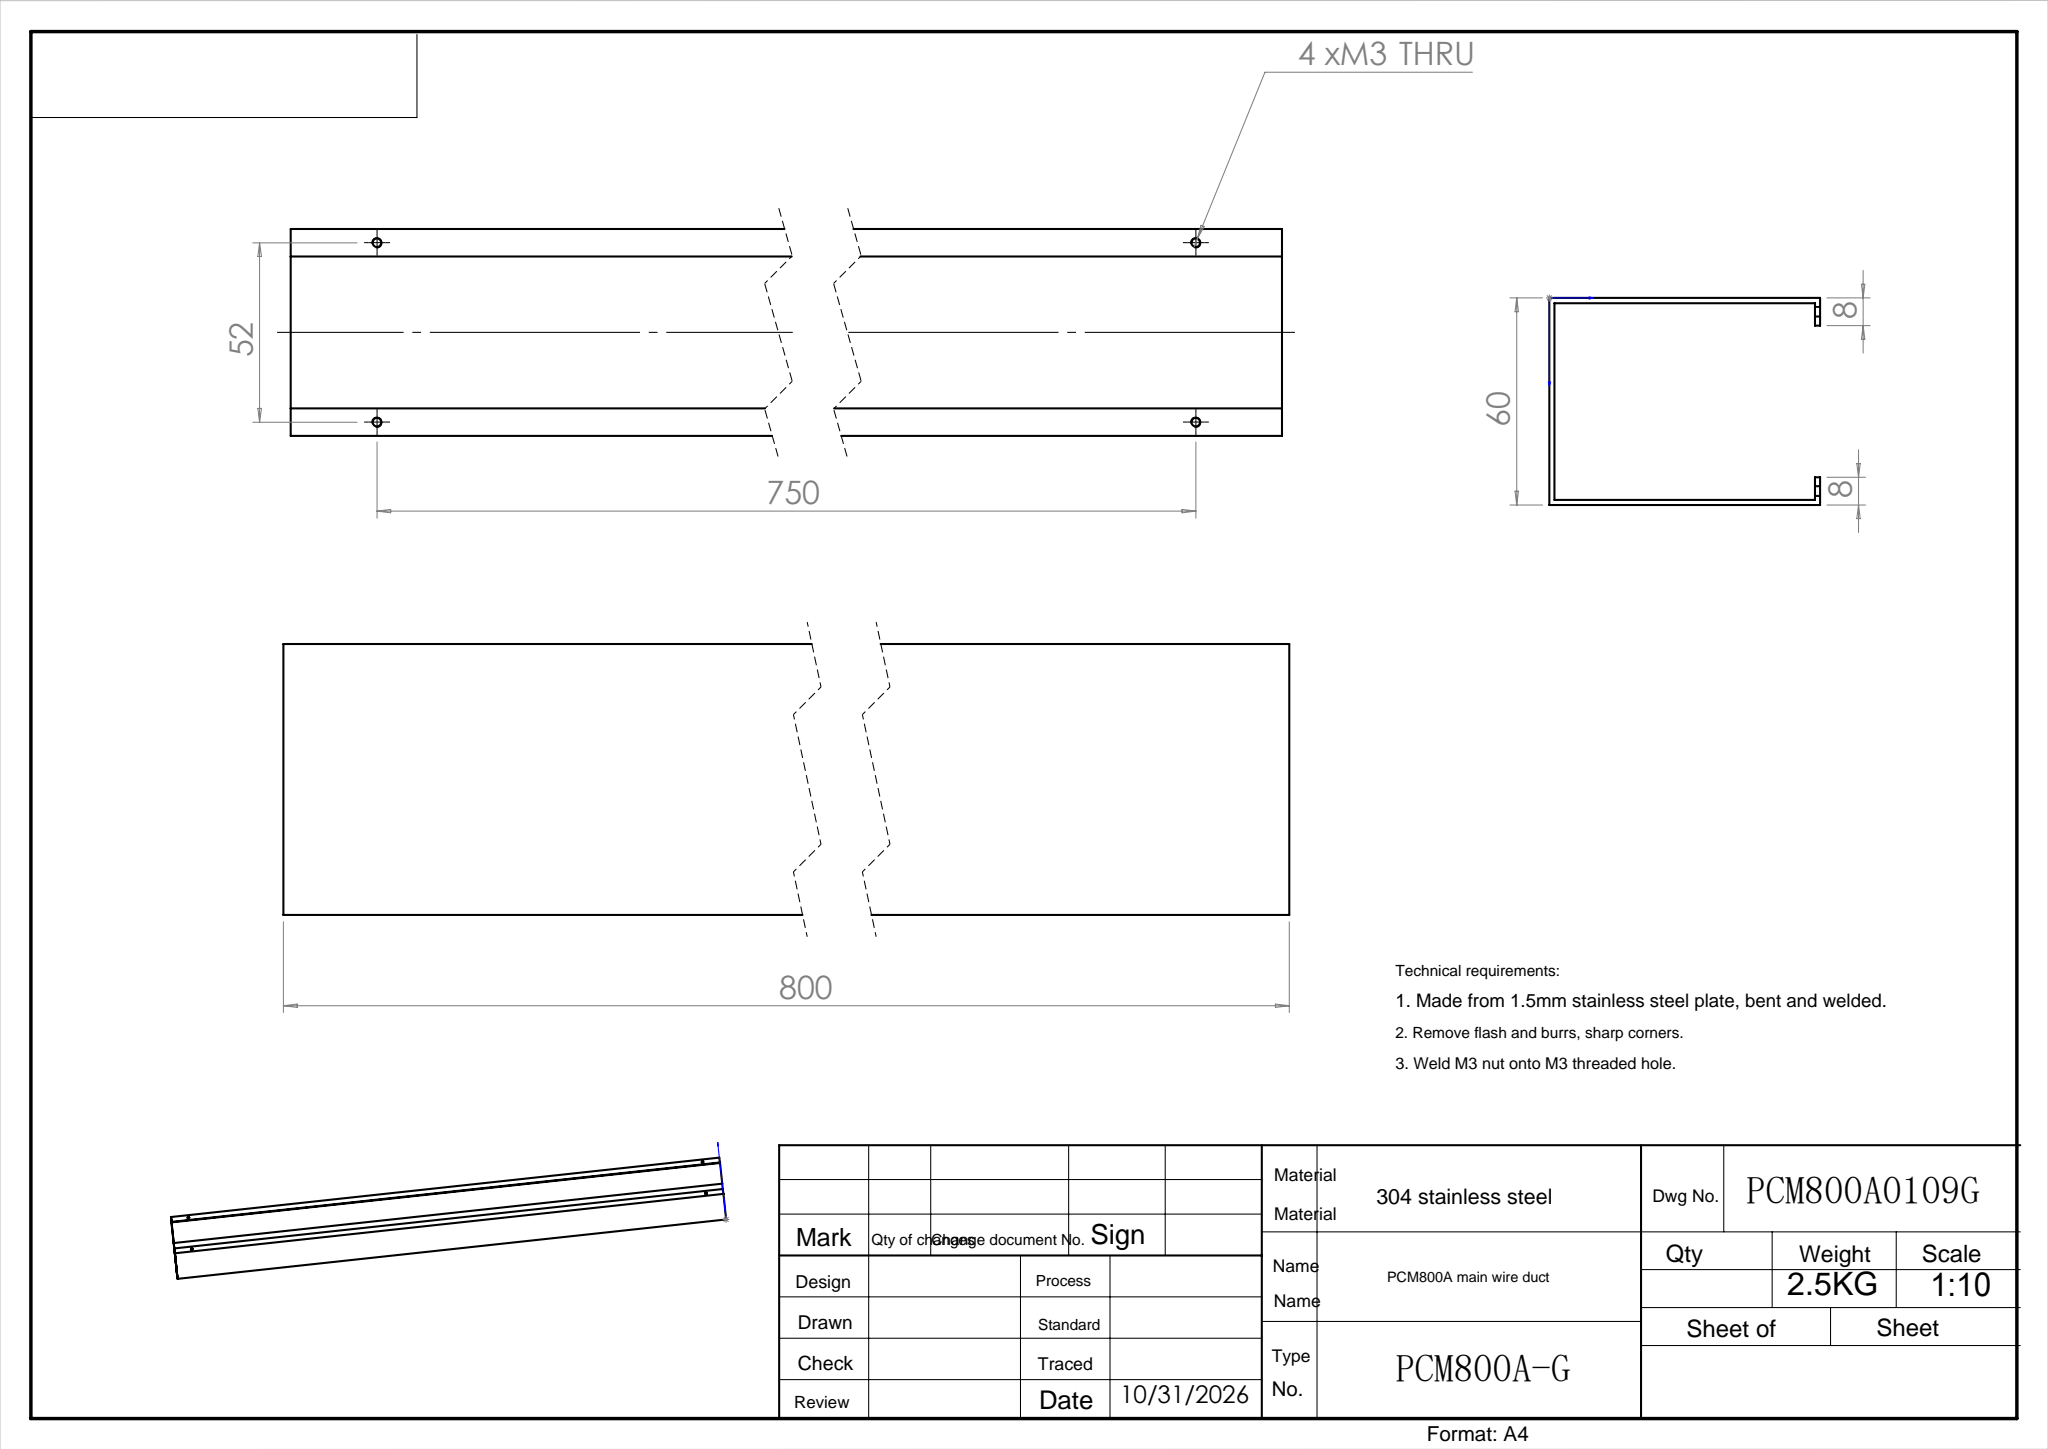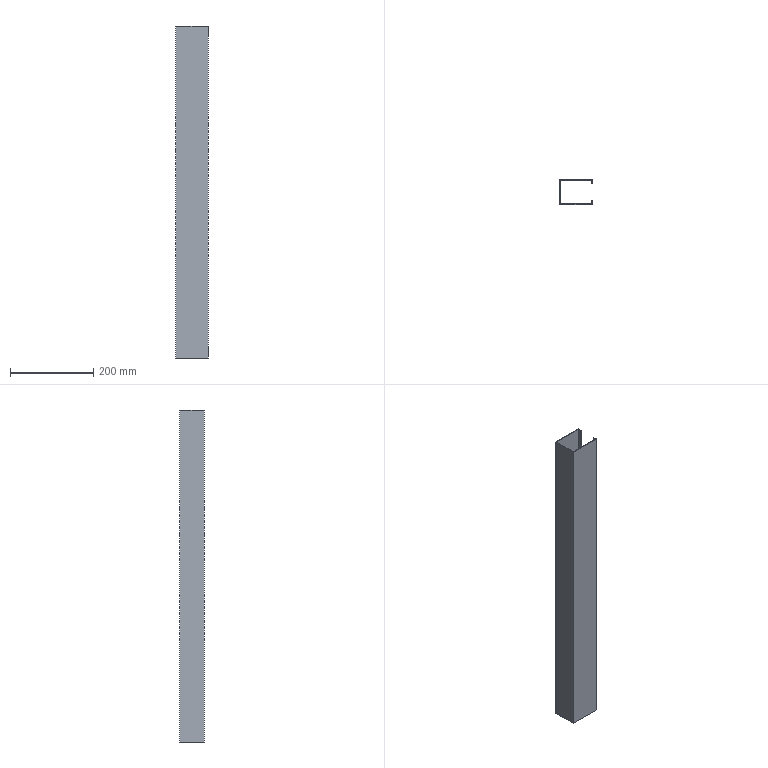Part | SolidWorks | features ExtruThin 1, HoleWzd 1, MirrorPattern 1 | 1 solid | 22 faces | box 78.5 x 60 x 800 mm | volume 272371 mm3 | plane 14 | cylinder 8 | commonest cylinder face diameters 2.5 x8
STEP:
#1=CARTESIAN_POINT('',(77.,4.,776.25));
#2=VERTEX_POINT('',#1);
#3=CARTESIAN_POINT('',(77.,4.,773.75));
#4=VERTEX_POINT('',#3);
#5=CARTESIAN_POINT('',(77.,4.,775.));
#6=DIRECTION('',(1.,0.,0.));
#7=DIRECTION('',(0.,0.,-1.));
#8=AXIS2_PLACEMENT_3D('',#5,#6,#7);
#9=CIRCLE('',#8,1.25);
#10=EDGE_CURVE('',#2,#4,#9,.T.);
#11=ORIENTED_EDGE('',*,*,#10,.F.);
#12=CARTESIAN_POINT('',(78.5,4.,776.25));
#13=VERTEX_POINT('',#12);
#14=CARTESIAN_POINT('',(78.5,4.,776.25));
#15=DIRECTION('',(1.,0.,0.));
#16=VECTOR('',#15,1000.);
#17=LINE('',#14,#16);
#18=EDGE_CURVE('',#2,#13,#17,.T.);
#19=ORIENTED_EDGE('',*,*,#18,.T.);
#20=CARTESIAN_POINT('',(78.5,4.,773.75));
#21=VERTEX_POINT('',#20);
#22=CARTESIAN_POINT('',(78.5,4.,775.));
#23=DIRECTION('',(1.,0.,0.));
#24=DIRECTION('',(0.,0.,-1.));
#25=AXIS2_PLACEMENT_3D('',#22,#23,#24);
#26=CIRCLE('',#25,1.25);
#27=EDGE_CURVE('',#13,#21,#26,.T.);
#28=ORIENTED_EDGE('',*,*,#27,.T.);
#29=CARTESIAN_POINT('',(78.5,4.,773.75));
#30=DIRECTION('',(1.,0.,0.));
#31=VECTOR('',#30,1000.);
#32=LINE('',#29,#31);
#33=EDGE_CURVE('',#4,#21,#32,.T.);
#34=ORIENTED_EDGE('',*,*,#33,.F.);
#35=EDGE_LOOP('',(#11,#19,#28,#34));
#36=FACE_OUTER_BOUND('',#35,.T.);
#37=CARTESIAN_POINT('',(78.5,4.,775.));
#38=DIRECTION('',(1.,0.,0.));
#39=DIRECTION('',(0.,0.,-1.));
#40=AXIS2_PLACEMENT_3D('',#37,#38,#39);
#41=CYLINDRICAL_SURFACE('',#40,1.25);
#42=ADVANCED_FACE('',(#36),#41,.F.);
#43=CARTESIAN_POINT('',(77.,4.,26.25));
#44=VERTEX_POINT('',#43);
#45=CARTESIAN_POINT('',(77.,4.,23.75));
#46=VERTEX_POINT('',#45);
#47=CARTESIAN_POINT('',(77.,4.,25.));
#48=DIRECTION('',(1.,0.,0.));
#49=DIRECTION('',(0.,0.,-1.));
#50=AXIS2_PLACEMENT_3D('',#47,#48,#49);
#51=CIRCLE('',#50,1.25);
#52=EDGE_CURVE('',#44,#46,#51,.T.);
#53=ORIENTED_EDGE('',*,*,#52,.F.);
#54=CARTESIAN_POINT('',(78.5,4.,26.25));
#55=VERTEX_POINT('',#54);
#56=CARTESIAN_POINT('',(78.5,4.,26.25));
#57=DIRECTION('',(1.,0.,0.));
#58=VECTOR('',#57,1000.);
#59=LINE('',#56,#58);
#60=EDGE_CURVE('',#44,#55,#59,.T.);
#61=ORIENTED_EDGE('',*,*,#60,.T.);
#62=CARTESIAN_POINT('',(78.5,4.,23.75));
#63=VERTEX_POINT('',#62);
#64=CARTESIAN_POINT('',(78.5,4.,25.));
#65=DIRECTION('',(1.,0.,0.));
#66=DIRECTION('',(0.,0.,-1.));
#67=AXIS2_PLACEMENT_3D('',#64,#65,#66);
#68=CIRCLE('',#67,1.25);
#69=EDGE_CURVE('',#55,#63,#68,.T.);
#70=ORIENTED_EDGE('',*,*,#69,.T.);
#71=CARTESIAN_POINT('',(78.5,4.,23.75));
#72=DIRECTION('',(1.,0.,0.));
#73=VECTOR('',#72,1000.);
#74=LINE('',#71,#73);
#75=EDGE_CURVE('',#46,#63,#74,.T.);
#76=ORIENTED_EDGE('',*,*,#75,.F.);
#77=EDGE_LOOP('',(#53,#61,#70,#76));
#78=FACE_OUTER_BOUND('',#77,.T.);
#79=CARTESIAN_POINT('',(78.5,4.,25.));
#80=DIRECTION('',(1.,0.,0.));
#81=DIRECTION('',(0.,0.,-1.));
#82=AXIS2_PLACEMENT_3D('',#79,#80,#81);
#83=CYLINDRICAL_SURFACE('',#82,1.25);
#84=ADVANCED_FACE('',(#78),#83,.F.);
#85=CARTESIAN_POINT('',(77.,56.,776.25));
#86=VERTEX_POINT('',#85);
#87=CARTESIAN_POINT('',(77.,56.,773.75));
#88=VERTEX_POINT('',#87);
#89=CARTESIAN_POINT('',(77.,56.,775.));
#90=DIRECTION('',(1.,0.,0.));
#91=DIRECTION('',(0.,1.,0.));
#92=AXIS2_PLACEMENT_3D('',#89,#90,#91);
#93=CIRCLE('',#92,1.25);
#94=EDGE_CURVE('',#86,#88,#93,.T.);
#95=ORIENTED_EDGE('',*,*,#94,.F.);
#96=CARTESIAN_POINT('',(78.5,56.,776.25));
#97=VERTEX_POINT('',#96);
#98=CARTESIAN_POINT('',(78.5,56.,776.25));
#99=DIRECTION('',(1.,0.,0.));
#100=VECTOR('',#99,1000.);
#101=LINE('',#98,#100);
#102=EDGE_CURVE('',#86,#97,#101,.T.);
#103=ORIENTED_EDGE('',*,*,#102,.T.);
#104=CARTESIAN_POINT('',(78.5,56.,773.75));
#105=VERTEX_POINT('',#104);
#106=CARTESIAN_POINT('',(78.5,56.,775.));
#107=DIRECTION('',(1.,0.,0.));
#108=DIRECTION('',(0.,0.,-1.));
#109=AXIS2_PLACEMENT_3D('',#106,#107,#108);
#110=CIRCLE('',#109,1.25);
#111=EDGE_CURVE('',#97,#105,#110,.T.);
#112=ORIENTED_EDGE('',*,*,#111,.T.);
#113=CARTESIAN_POINT('',(78.5,56.,773.75));
#114=DIRECTION('',(1.,0.,0.));
#115=VECTOR('',#114,1000.);
#116=LINE('',#113,#115);
#117=EDGE_CURVE('',#88,#105,#116,.T.);
#118=ORIENTED_EDGE('',*,*,#117,.F.);
#119=EDGE_LOOP('',(#95,#103,#112,#118));
#120=FACE_OUTER_BOUND('',#119,.T.);
#121=CARTESIAN_POINT('',(78.5,56.,775.));
#122=DIRECTION('',(1.,0.,0.));
#123=DIRECTION('',(0.,0.,-1.));
#124=AXIS2_PLACEMENT_3D('',#121,#122,#123);
#125=CYLINDRICAL_SURFACE('',#124,1.25);
#126=ADVANCED_FACE('',(#120),#125,.F.);
#127=CARTESIAN_POINT('',(77.,56.,26.25));
#128=VERTEX_POINT('',#127);
#129=CARTESIAN_POINT('',(77.,56.,23.75));
#130=VERTEX_POINT('',#129);
#131=CARTESIAN_POINT('',(77.,56.,25.));
#132=DIRECTION('',(1.,0.,0.));
#133=DIRECTION('',(0.,1.,0.));
#134=AXIS2_PLACEMENT_3D('',#131,#132,#133);
#135=CIRCLE('',#134,1.25);
#136=EDGE_CURVE('',#128,#130,#135,.T.);
#137=ORIENTED_EDGE('',*,*,#136,.F.);
#138=CARTESIAN_POINT('',(78.5,56.,26.25));
#139=VERTEX_POINT('',#138);
#140=CARTESIAN_POINT('',(78.5,56.,26.25));
#141=DIRECTION('',(1.,0.,0.));
#142=VECTOR('',#141,1000.);
#143=LINE('',#140,#142);
#144=EDGE_CURVE('',#128,#139,#143,.T.);
#145=ORIENTED_EDGE('',*,*,#144,.T.);
#146=CARTESIAN_POINT('',(78.5,56.,23.75));
#147=VERTEX_POINT('',#146);
#148=CARTESIAN_POINT('',(78.5,56.,25.));
#149=DIRECTION('',(1.,0.,0.));
#150=DIRECTION('',(0.,0.,-1.));
#151=AXIS2_PLACEMENT_3D('',#148,#149,#150);
#152=CIRCLE('',#151,1.25);
#153=EDGE_CURVE('',#139,#147,#152,.T.);
#154=ORIENTED_EDGE('',*,*,#153,.T.);
#155=CARTESIAN_POINT('',(78.5,56.,23.75));
#156=DIRECTION('',(1.,0.,0.));
#157=VECTOR('',#156,1000.);
#158=LINE('',#155,#157);
#159=EDGE_CURVE('',#130,#147,#158,.T.);
#160=ORIENTED_EDGE('',*,*,#159,.F.);
#161=EDGE_LOOP('',(#137,#145,#154,#160));
#162=FACE_OUTER_BOUND('',#161,.T.);
#163=CARTESIAN_POINT('',(78.5,56.,25.));
#164=DIRECTION('',(1.,0.,0.));
#165=DIRECTION('',(0.,0.,-1.));
#166=AXIS2_PLACEMENT_3D('',#163,#164,#165);
#167=CYLINDRICAL_SURFACE('',#166,1.25);
#168=ADVANCED_FACE('',(#162),#167,.F.);
#169=CARTESIAN_POINT('',(77.,56.,775.));
#170=DIRECTION('',(1.,0.,0.));
#171=DIRECTION('',(0.,1.,0.));
#172=AXIS2_PLACEMENT_3D('',#169,#170,#171);
#173=CIRCLE('',#172,1.25);
#174=EDGE_CURVE('',#88,#86,#173,.T.);
#175=ORIENTED_EDGE('',*,*,#174,.T.);
#176=ORIENTED_EDGE('',*,*,#94,.T.);
#177=EDGE_LOOP('',(#175,#176));
#178=FACE_BOUND('',#177,.T.);
#179=CARTESIAN_POINT('',(77.,56.,25.));
#180=DIRECTION('',(1.,0.,0.));
#181=DIRECTION('',(0.,1.,0.));
#182=AXIS2_PLACEMENT_3D('',#179,#180,#181);
#183=CIRCLE('',#182,1.25);
#184=EDGE_CURVE('',#130,#128,#183,.T.);
#185=ORIENTED_EDGE('',*,*,#184,.T.);
#186=ORIENTED_EDGE('',*,*,#136,.T.);
#187=EDGE_LOOP('',(#185,#186));
#188=FACE_BOUND('',#187,.T.);
#189=CARTESIAN_POINT('',(77.,58.5,0.));
#190=VERTEX_POINT('',#189);
#191=CARTESIAN_POINT('',(77.,52.,0.));
#192=VERTEX_POINT('',#191);
#193=CARTESIAN_POINT('',(77.,60.,0.));
#194=DIRECTION('',(0.,-1.,0.));
#195=VECTOR('',#194,1000.);
#196=LINE('',#193,#195);
#197=EDGE_CURVE('',#190,#192,#196,.T.);
#198=ORIENTED_EDGE('',*,*,#197,.T.);
#199=CARTESIAN_POINT('',(77.,52.,800.));
#200=VERTEX_POINT('',#199);
#201=CARTESIAN_POINT('',(77.,52.,800.));
#202=DIRECTION('',(0.,0.,-1.));
#203=VECTOR('',#202,1000.);
#204=LINE('',#201,#203);
#205=EDGE_CURVE('',#200,#192,#204,.T.);
#206=ORIENTED_EDGE('',*,*,#205,.F.);
#207=CARTESIAN_POINT('',(77.,58.5,800.));
#208=VERTEX_POINT('',#207);
#209=CARTESIAN_POINT('',(77.,60.,800.));
#210=DIRECTION('',(0.,-1.,0.));
#211=VECTOR('',#210,1000.);
#212=LINE('',#209,#211);
#213=EDGE_CURVE('',#208,#200,#212,.T.);
#214=ORIENTED_EDGE('',*,*,#213,.F.);
#215=CARTESIAN_POINT('',(77.,58.5,800.));
#216=DIRECTION('',(0.,0.,-1.));
#217=VECTOR('',#216,1000.);
#218=LINE('',#215,#217);
#219=EDGE_CURVE('',#208,#190,#218,.T.);
#220=ORIENTED_EDGE('',*,*,#219,.T.);
#221=EDGE_LOOP('',(#198,#206,#214,#220));
#222=FACE_OUTER_BOUND('',#221,.T.);
#223=CARTESIAN_POINT('',(77.,60.,800.));
#224=DIRECTION('',(1.,0.,0.));
#225=DIRECTION('',(0.,1.,0.));
#226=AXIS2_PLACEMENT_3D('',#223,#224,#225);
#227=PLANE('',#226);
#228=ADVANCED_FACE('',(#178,#188,#222),#227,.F.);
#229=CARTESIAN_POINT('',(78.5,52.,0.));
#230=VERTEX_POINT('',#229);
#231=CARTESIAN_POINT('',(78.5,52.,0.));
#232=DIRECTION('',(-1.,0.,0.));
#233=VECTOR('',#232,1000.);
#234=LINE('',#231,#233);
#235=EDGE_CURVE('',#230,#192,#234,.T.);
#236=ORIENTED_EDGE('',*,*,#235,.F.);
#237=CARTESIAN_POINT('',(78.5,52.,800.));
#238=VERTEX_POINT('',#237);
#239=CARTESIAN_POINT('',(78.5,52.,800.));
#240=DIRECTION('',(0.,0.,-1.));
#241=VECTOR('',#240,1000.);
#242=LINE('',#239,#241);
#243=EDGE_CURVE('',#238,#230,#242,.T.);
#244=ORIENTED_EDGE('',*,*,#243,.F.);
#245=CARTESIAN_POINT('',(78.5,52.,800.));
#246=DIRECTION('',(-1.,0.,0.));
#247=VECTOR('',#246,1000.);
#248=LINE('',#245,#247);
#249=EDGE_CURVE('',#238,#200,#248,.T.);
#250=ORIENTED_EDGE('',*,*,#249,.T.);
#251=ORIENTED_EDGE('',*,*,#205,.T.);
#252=EDGE_LOOP('',(#236,#244,#250,#251));
#253=FACE_OUTER_BOUND('',#252,.T.);
#254=CARTESIAN_POINT('',(78.5,52.,800.));
#255=DIRECTION('',(0.,-1.,0.));
#256=DIRECTION('',(1.,0.,0.));
#257=AXIS2_PLACEMENT_3D('',#254,#255,#256);
#258=PLANE('',#257);
#259=ADVANCED_FACE('',(#253),#258,.T.);
#260=CARTESIAN_POINT('',(78.5,56.,775.));
#261=DIRECTION('',(1.,0.,0.));
#262=DIRECTION('',(0.,0.,-1.));
#263=AXIS2_PLACEMENT_3D('',#260,#261,#262);
#264=CIRCLE('',#263,1.25);
#265=EDGE_CURVE('',#105,#97,#264,.T.);
#266=ORIENTED_EDGE('',*,*,#265,.F.);
#267=ORIENTED_EDGE('',*,*,#111,.F.);
#268=EDGE_LOOP('',(#266,#267));
#269=FACE_BOUND('',#268,.T.);
#270=CARTESIAN_POINT('',(78.5,56.,25.));
#271=DIRECTION('',(1.,0.,0.));
#272=DIRECTION('',(0.,0.,-1.));
#273=AXIS2_PLACEMENT_3D('',#270,#271,#272);
#274=CIRCLE('',#273,1.25);
#275=EDGE_CURVE('',#147,#139,#274,.T.);
#276=ORIENTED_EDGE('',*,*,#275,.F.);
#277=ORIENTED_EDGE('',*,*,#153,.F.);
#278=EDGE_LOOP('',(#276,#277));
#279=FACE_BOUND('',#278,.T.);
#280=CARTESIAN_POINT('',(78.5,60.,0.));
#281=VERTEX_POINT('',#280);
#282=CARTESIAN_POINT('',(78.5,60.,0.));
#283=DIRECTION('',(0.,-1.,0.));
#284=VECTOR('',#283,1000.);
#285=LINE('',#282,#284);
#286=EDGE_CURVE('',#281,#230,#285,.T.);
#287=ORIENTED_EDGE('',*,*,#286,.F.);
#288=CARTESIAN_POINT('',(78.5,60.,800.));
#289=VERTEX_POINT('',#288);
#290=CARTESIAN_POINT('',(78.5,60.,800.));
#291=DIRECTION('',(0.,0.,-1.));
#292=VECTOR('',#291,1000.);
#293=LINE('',#290,#292);
#294=EDGE_CURVE('',#289,#281,#293,.T.);
#295=ORIENTED_EDGE('',*,*,#294,.F.);
#296=CARTESIAN_POINT('',(78.5,60.,800.));
#297=DIRECTION('',(0.,-1.,0.));
#298=VECTOR('',#297,1000.);
#299=LINE('',#296,#298);
#300=EDGE_CURVE('',#289,#238,#299,.T.);
#301=ORIENTED_EDGE('',*,*,#300,.T.);
#302=ORIENTED_EDGE('',*,*,#243,.T.);
#303=EDGE_LOOP('',(#287,#295,#301,#302));
#304=FACE_OUTER_BOUND('',#303,.T.);
#305=CARTESIAN_POINT('',(78.5,60.,800.));
#306=DIRECTION('',(1.,0.,0.));
#307=DIRECTION('',(0.,1.,0.));
#308=AXIS2_PLACEMENT_3D('',#305,#306,#307);
#309=PLANE('',#308);
#310=ADVANCED_FACE('',(#269,#279,#304),#309,.T.);
#311=CARTESIAN_POINT('',(0.,60.,0.));
#312=VERTEX_POINT('',#311);
#313=CARTESIAN_POINT('',(0.,60.,0.));
#314=DIRECTION('',(1.,0.,0.));
#315=VECTOR('',#314,1000.);
#316=LINE('',#313,#315);
#317=EDGE_CURVE('',#312,#281,#316,.T.);
#318=ORIENTED_EDGE('',*,*,#317,.F.);
#319=CARTESIAN_POINT('',(0.,60.,800.));
#320=VERTEX_POINT('',#319);
#321=CARTESIAN_POINT('',(0.,60.,800.));
#322=DIRECTION('',(0.,0.,-1.));
#323=VECTOR('',#322,1000.);
#324=LINE('',#321,#323);
#325=EDGE_CURVE('',#320,#312,#324,.T.);
#326=ORIENTED_EDGE('',*,*,#325,.F.);
#327=CARTESIAN_POINT('',(0.,60.,800.));
#328=DIRECTION('',(1.,0.,0.));
#329=VECTOR('',#328,1000.);
#330=LINE('',#327,#329);
#331=EDGE_CURVE('',#320,#289,#330,.T.);
#332=ORIENTED_EDGE('',*,*,#331,.T.);
#333=ORIENTED_EDGE('',*,*,#294,.T.);
#334=EDGE_LOOP('',(#318,#326,#332,#333));
#335=FACE_OUTER_BOUND('',#334,.T.);
#336=CARTESIAN_POINT('',(0.,60.,800.));
#337=DIRECTION('',(0.,1.,0.));
#338=DIRECTION('',(0.,0.,1.));
#339=AXIS2_PLACEMENT_3D('',#336,#337,#338);
#340=PLANE('',#339);
#341=ADVANCED_FACE('',(#335),#340,.T.);
#342=CARTESIAN_POINT('',(0.,0.,0.));
#343=VERTEX_POINT('',#342);
#344=CARTESIAN_POINT('',(0.,0.,0.));
#345=DIRECTION('',(0.,1.,0.));
#346=VECTOR('',#345,1000.);
#347=LINE('',#344,#346);
#348=EDGE_CURVE('',#343,#312,#347,.T.);
#349=ORIENTED_EDGE('',*,*,#348,.F.);
#350=CARTESIAN_POINT('',(0.,0.,800.));
#351=VERTEX_POINT('',#350);
#352=CARTESIAN_POINT('',(0.,0.,800.));
#353=DIRECTION('',(0.,0.,-1.));
#354=VECTOR('',#353,1000.);
#355=LINE('',#352,#354);
#356=EDGE_CURVE('',#351,#343,#355,.T.);
#357=ORIENTED_EDGE('',*,*,#356,.F.);
#358=CARTESIAN_POINT('',(0.,0.,800.));
#359=DIRECTION('',(0.,1.,0.));
#360=VECTOR('',#359,1000.);
#361=LINE('',#358,#360);
#362=EDGE_CURVE('',#351,#320,#361,.T.);
#363=ORIENTED_EDGE('',*,*,#362,.T.);
#364=ORIENTED_EDGE('',*,*,#325,.T.);
#365=EDGE_LOOP('',(#349,#357,#363,#364));
#366=FACE_OUTER_BOUND('',#365,.T.);
#367=CARTESIAN_POINT('',(0.,0.,800.));
#368=DIRECTION('',(-1.,0.,0.));
#369=DIRECTION('',(0.,0.,1.));
#370=AXIS2_PLACEMENT_3D('',#367,#368,#369);
#371=PLANE('',#370);
#372=ADVANCED_FACE('',(#366),#371,.T.);
#373=CARTESIAN_POINT('',(78.5,0.,0.));
#374=VERTEX_POINT('',#373);
#375=CARTESIAN_POINT('',(0.,0.,0.));
#376=DIRECTION('',(-1.,0.,0.));
#377=VECTOR('',#376,1000.);
#378=LINE('',#375,#377);
#379=EDGE_CURVE('',#374,#343,#378,.T.);
#380=ORIENTED_EDGE('',*,*,#379,.F.);
#381=CARTESIAN_POINT('',(78.5,0.,800.));
#382=VERTEX_POINT('',#381);
#383=CARTESIAN_POINT('',(78.5,0.,800.));
#384=DIRECTION('',(0.,0.,-1.));
#385=VECTOR('',#384,1000.);
#386=LINE('',#383,#385);
#387=EDGE_CURVE('',#382,#374,#386,.T.);
#388=ORIENTED_EDGE('',*,*,#387,.F.);
#389=CARTESIAN_POINT('',(0.,0.,800.));
#390=DIRECTION('',(-1.,0.,0.));
#391=VECTOR('',#390,1000.);
#392=LINE('',#389,#391);
#393=EDGE_CURVE('',#382,#351,#392,.T.);
#394=ORIENTED_EDGE('',*,*,#393,.T.);
#395=ORIENTED_EDGE('',*,*,#356,.T.);
#396=EDGE_LOOP('',(#380,#388,#394,#395));
#397=FACE_OUTER_BOUND('',#396,.T.);
#398=CARTESIAN_POINT('',(0.,0.,800.));
#399=DIRECTION('',(0.,-1.,0.));
#400=DIRECTION('',(0.,0.,-1.));
#401=AXIS2_PLACEMENT_3D('',#398,#399,#400);
#402=PLANE('',#401);
#403=ADVANCED_FACE('',(#397),#402,.T.);
#404=CARTESIAN_POINT('',(78.5,4.,775.));
#405=DIRECTION('',(1.,0.,0.));
#406=DIRECTION('',(0.,0.,-1.));
#407=AXIS2_PLACEMENT_3D('',#404,#405,#406);
#408=CIRCLE('',#407,1.25);
#409=EDGE_CURVE('',#21,#13,#408,.T.);
#410=ORIENTED_EDGE('',*,*,#409,.F.);
#411=ORIENTED_EDGE('',*,*,#27,.F.);
#412=EDGE_LOOP('',(#410,#411));
#413=FACE_BOUND('',#412,.T.);
#414=CARTESIAN_POINT('',(78.5,4.,25.));
#415=DIRECTION('',(1.,0.,0.));
#416=DIRECTION('',(0.,0.,-1.));
#417=AXIS2_PLACEMENT_3D('',#414,#415,#416);
#418=CIRCLE('',#417,1.25);
#419=EDGE_CURVE('',#63,#55,#418,.T.);
#420=ORIENTED_EDGE('',*,*,#419,.F.);
#421=ORIENTED_EDGE('',*,*,#69,.F.);
#422=EDGE_LOOP('',(#420,#421));
#423=FACE_BOUND('',#422,.T.);
#424=CARTESIAN_POINT('',(78.5,8.,0.));
#425=VERTEX_POINT('',#424);
#426=CARTESIAN_POINT('',(78.5,0.,0.));
#427=DIRECTION('',(0.,-1.,0.));
#428=VECTOR('',#427,1000.);
#429=LINE('',#426,#428);
#430=EDGE_CURVE('',#425,#374,#429,.T.);
#431=ORIENTED_EDGE('',*,*,#430,.F.);
#432=CARTESIAN_POINT('',(78.5,8.,800.));
#433=VERTEX_POINT('',#432);
#434=CARTESIAN_POINT('',(78.5,8.,800.));
#435=DIRECTION('',(0.,0.,-1.));
#436=VECTOR('',#435,1000.);
#437=LINE('',#434,#436);
#438=EDGE_CURVE('',#433,#425,#437,.T.);
#439=ORIENTED_EDGE('',*,*,#438,.F.);
#440=CARTESIAN_POINT('',(78.5,0.,800.));
#441=DIRECTION('',(0.,-1.,0.));
#442=VECTOR('',#441,1000.);
#443=LINE('',#440,#442);
#444=EDGE_CURVE('',#433,#382,#443,.T.);
#445=ORIENTED_EDGE('',*,*,#444,.T.);
#446=ORIENTED_EDGE('',*,*,#387,.T.);
#447=EDGE_LOOP('',(#431,#439,#445,#446));
#448=FACE_OUTER_BOUND('',#447,.T.);
#449=CARTESIAN_POINT('',(78.5,0.,800.));
#450=DIRECTION('',(1.,0.,0.));
#451=DIRECTION('',(0.,0.,-1.));
#452=AXIS2_PLACEMENT_3D('',#449,#450,#451);
#453=PLANE('',#452);
#454=ADVANCED_FACE('',(#413,#423,#448),#453,.T.);
#455=CARTESIAN_POINT('',(77.,8.,0.));
#456=VERTEX_POINT('',#455);
#457=CARTESIAN_POINT('',(77.,8.,0.));
#458=DIRECTION('',(1.,0.,0.));
#459=VECTOR('',#458,1000.);
#460=LINE('',#457,#459);
#461=EDGE_CURVE('',#456,#425,#460,.T.);
#462=ORIENTED_EDGE('',*,*,#461,.F.);
#463=CARTESIAN_POINT('',(77.,8.,800.));
#464=VERTEX_POINT('',#463);
#465=CARTESIAN_POINT('',(77.,8.,800.));
#466=DIRECTION('',(0.,0.,-1.));
#467=VECTOR('',#466,1000.);
#468=LINE('',#465,#467);
#469=EDGE_CURVE('',#464,#456,#468,.T.);
#470=ORIENTED_EDGE('',*,*,#469,.F.);
#471=CARTESIAN_POINT('',(77.,8.,800.));
#472=DIRECTION('',(1.,0.,0.));
#473=VECTOR('',#472,1000.);
#474=LINE('',#471,#473);
#475=EDGE_CURVE('',#464,#433,#474,.T.);
#476=ORIENTED_EDGE('',*,*,#475,.T.);
#477=ORIENTED_EDGE('',*,*,#438,.T.);
#478=EDGE_LOOP('',(#462,#470,#476,#477));
#479=FACE_OUTER_BOUND('',#478,.T.);
#480=CARTESIAN_POINT('',(77.,8.,800.));
#481=DIRECTION('',(0.,1.,0.));
#482=DIRECTION('',(0.,0.,1.));
#483=AXIS2_PLACEMENT_3D('',#480,#481,#482);
#484=PLANE('',#483);
#485=ADVANCED_FACE('',(#479),#484,.T.);
#486=CARTESIAN_POINT('',(77.,4.,775.));
#487=DIRECTION('',(1.,0.,0.));
#488=DIRECTION('',(0.,0.,-1.));
#489=AXIS2_PLACEMENT_3D('',#486,#487,#488);
#490=CIRCLE('',#489,1.25);
#491=EDGE_CURVE('',#4,#2,#490,.T.);
#492=ORIENTED_EDGE('',*,*,#491,.T.);
#493=ORIENTED_EDGE('',*,*,#10,.T.);
#494=EDGE_LOOP('',(#492,#493));
#495=FACE_BOUND('',#494,.T.);
#496=CARTESIAN_POINT('',(77.,4.,25.));
#497=DIRECTION('',(1.,0.,0.));
#498=DIRECTION('',(0.,0.,-1.));
#499=AXIS2_PLACEMENT_3D('',#496,#497,#498);
#500=CIRCLE('',#499,1.25);
#501=EDGE_CURVE('',#46,#44,#500,.T.);
#502=ORIENTED_EDGE('',*,*,#501,.T.);
#503=ORIENTED_EDGE('',*,*,#52,.T.);
#504=EDGE_LOOP('',(#502,#503));
#505=FACE_BOUND('',#504,.T.);
#506=CARTESIAN_POINT('',(77.,1.5,0.));
#507=VERTEX_POINT('',#506);
#508=CARTESIAN_POINT('',(77.,0.,0.));
#509=DIRECTION('',(0.,-1.,0.));
#510=VECTOR('',#509,1000.);
#511=LINE('',#508,#510);
#512=EDGE_CURVE('',#456,#507,#511,.T.);
#513=ORIENTED_EDGE('',*,*,#512,.T.);
#514=CARTESIAN_POINT('',(77.,1.5,800.));
#515=VERTEX_POINT('',#514);
#516=CARTESIAN_POINT('',(77.,1.5,800.));
#517=DIRECTION('',(0.,0.,-1.));
#518=VECTOR('',#517,1000.);
#519=LINE('',#516,#518);
#520=EDGE_CURVE('',#515,#507,#519,.T.);
#521=ORIENTED_EDGE('',*,*,#520,.F.);
#522=CARTESIAN_POINT('',(77.,0.,800.));
#523=DIRECTION('',(0.,-1.,0.));
#524=VECTOR('',#523,1000.);
#525=LINE('',#522,#524);
#526=EDGE_CURVE('',#464,#515,#525,.T.);
#527=ORIENTED_EDGE('',*,*,#526,.F.);
#528=ORIENTED_EDGE('',*,*,#469,.T.);
#529=EDGE_LOOP('',(#513,#521,#527,#528));
#530=FACE_OUTER_BOUND('',#529,.T.);
#531=CARTESIAN_POINT('',(77.,0.,800.));
#532=DIRECTION('',(1.,0.,0.));
#533=DIRECTION('',(0.,0.,-1.));
#534=AXIS2_PLACEMENT_3D('',#531,#532,#533);
#535=PLANE('',#534);
#536=ADVANCED_FACE('',(#495,#505,#530),#535,.F.);
#537=CARTESIAN_POINT('',(1.5,1.5,0.));
#538=VERTEX_POINT('',#537);
#539=CARTESIAN_POINT('',(0.,1.5,0.));
#540=DIRECTION('',(-1.,0.,0.));
#541=VECTOR('',#540,1000.);
#542=LINE('',#539,#541);
#543=EDGE_CURVE('',#507,#538,#542,.T.);
#544=ORIENTED_EDGE('',*,*,#543,.T.);
#545=CARTESIAN_POINT('',(1.5,1.5,800.));
#546=VERTEX_POINT('',#545);
#547=CARTESIAN_POINT('',(1.5,1.5,800.));
#548=DIRECTION('',(0.,0.,-1.));
#549=VECTOR('',#548,1000.);
#550=LINE('',#547,#549);
#551=EDGE_CURVE('',#546,#538,#550,.T.);
#552=ORIENTED_EDGE('',*,*,#551,.F.);
#553=CARTESIAN_POINT('',(0.,1.5,800.));
#554=DIRECTION('',(-1.,0.,0.));
#555=VECTOR('',#554,1000.);
#556=LINE('',#553,#555);
#557=EDGE_CURVE('',#515,#546,#556,.T.);
#558=ORIENTED_EDGE('',*,*,#557,.F.);
#559=ORIENTED_EDGE('',*,*,#520,.T.);
#560=EDGE_LOOP('',(#544,#552,#558,#559));
#561=FACE_OUTER_BOUND('',#560,.T.);
#562=CARTESIAN_POINT('',(0.,1.5,800.));
#563=DIRECTION('',(0.,-1.,0.));
#564=DIRECTION('',(0.,0.,-1.));
#565=AXIS2_PLACEMENT_3D('',#562,#563,#564);
#566=PLANE('',#565);
#567=ADVANCED_FACE('',(#561),#566,.F.);
#568=CARTESIAN_POINT('',(1.5,58.5,0.));
#569=VERTEX_POINT('',#568);
#570=CARTESIAN_POINT('',(1.5,0.,0.));
#571=DIRECTION('',(0.,1.,0.));
#572=VECTOR('',#571,1000.);
#573=LINE('',#570,#572);
#574=EDGE_CURVE('',#538,#569,#573,.T.);
#575=ORIENTED_EDGE('',*,*,#574,.T.);
#576=CARTESIAN_POINT('',(1.5,58.5,800.));
#577=VERTEX_POINT('',#576);
#578=CARTESIAN_POINT('',(1.5,58.5,800.));
#579=DIRECTION('',(0.,0.,-1.));
#580=VECTOR('',#579,1000.);
#581=LINE('',#578,#580);
#582=EDGE_CURVE('',#577,#569,#581,.T.);
#583=ORIENTED_EDGE('',*,*,#582,.F.);
#584=CARTESIAN_POINT('',(1.5,0.,800.));
#585=DIRECTION('',(0.,1.,0.));
#586=VECTOR('',#585,1000.);
#587=LINE('',#584,#586);
#588=EDGE_CURVE('',#546,#577,#587,.T.);
#589=ORIENTED_EDGE('',*,*,#588,.F.);
#590=ORIENTED_EDGE('',*,*,#551,.T.);
#591=EDGE_LOOP('',(#575,#583,#589,#590));
#592=FACE_OUTER_BOUND('',#591,.T.);
#593=CARTESIAN_POINT('',(1.5,0.,800.));
#594=DIRECTION('',(-1.,0.,0.));
#595=DIRECTION('',(0.,0.,1.));
#596=AXIS2_PLACEMENT_3D('',#593,#594,#595);
#597=PLANE('',#596);
#598=ADVANCED_FACE('',(#592),#597,.F.);
#599=CARTESIAN_POINT('',(0.,58.5,0.));
#600=DIRECTION('',(1.,0.,0.));
#601=VECTOR('',#600,1000.);
#602=LINE('',#599,#601);
#603=EDGE_CURVE('',#569,#190,#602,.T.);
#604=ORIENTED_EDGE('',*,*,#603,.T.);
#605=ORIENTED_EDGE('',*,*,#219,.F.);
#606=CARTESIAN_POINT('',(0.,58.5,800.));
#607=DIRECTION('',(1.,0.,0.));
#608=VECTOR('',#607,1000.);
#609=LINE('',#606,#608);
#610=EDGE_CURVE('',#577,#208,#609,.T.);
#611=ORIENTED_EDGE('',*,*,#610,.F.);
#612=ORIENTED_EDGE('',*,*,#582,.T.);
#613=EDGE_LOOP('',(#604,#605,#611,#612));
#614=FACE_OUTER_BOUND('',#613,.T.);
#615=CARTESIAN_POINT('',(0.,58.5,800.));
#616=DIRECTION('',(0.,1.,0.));
#617=DIRECTION('',(0.,0.,1.));
#618=AXIS2_PLACEMENT_3D('',#615,#616,#617);
#619=PLANE('',#618);
#620=ADVANCED_FACE('',(#614),#619,.F.);
#621=ORIENTED_EDGE('',*,*,#213,.T.);
#622=ORIENTED_EDGE('',*,*,#249,.F.);
#623=ORIENTED_EDGE('',*,*,#300,.F.);
#624=ORIENTED_EDGE('',*,*,#331,.F.);
#625=ORIENTED_EDGE('',*,*,#362,.F.);
#626=ORIENTED_EDGE('',*,*,#393,.F.);
#627=ORIENTED_EDGE('',*,*,#444,.F.);
#628=ORIENTED_EDGE('',*,*,#475,.F.);
#629=ORIENTED_EDGE('',*,*,#526,.T.);
#630=ORIENTED_EDGE('',*,*,#557,.T.);
#631=ORIENTED_EDGE('',*,*,#588,.T.);
#632=ORIENTED_EDGE('',*,*,#610,.T.);
#633=EDGE_LOOP('',(#621,#622,#623,#624,#625,#626,#627,#628,#629,#630,#631,#632));
#634=FACE_OUTER_BOUND('',#633,.T.);
#635=CARTESIAN_POINT('',(77.,52.,800.));
#636=DIRECTION('',(0.,0.,-1.));
#637=DIRECTION('',(-1.,0.,0.));
#638=AXIS2_PLACEMENT_3D('',#635,#636,#637);
#639=PLANE('',#638);
#640=ADVANCED_FACE('',(#634),#639,.F.);
#641=ORIENTED_EDGE('',*,*,#197,.F.);
#642=ORIENTED_EDGE('',*,*,#603,.F.);
#643=ORIENTED_EDGE('',*,*,#574,.F.);
#644=ORIENTED_EDGE('',*,*,#543,.F.);
#645=ORIENTED_EDGE('',*,*,#512,.F.);
#646=ORIENTED_EDGE('',*,*,#461,.T.);
#647=ORIENTED_EDGE('',*,*,#430,.T.);
#648=ORIENTED_EDGE('',*,*,#379,.T.);
#649=ORIENTED_EDGE('',*,*,#348,.T.);
#650=ORIENTED_EDGE('',*,*,#317,.T.);
#651=ORIENTED_EDGE('',*,*,#286,.T.);
#652=ORIENTED_EDGE('',*,*,#235,.T.);
#653=EDGE_LOOP('',(#641,#642,#643,#644,#645,#646,#647,#648,#649,#650,#651,#652));
#654=FACE_OUTER_BOUND('',#653,.T.);
#655=CARTESIAN_POINT('',(77.,52.,0.));
#656=DIRECTION('',(0.,0.,-1.));
#657=DIRECTION('',(-1.,0.,0.));
#658=AXIS2_PLACEMENT_3D('',#655,#656,#657);
#659=PLANE('',#658);
#660=ADVANCED_FACE('',(#654),#659,.T.);
#661=ORIENTED_EDGE('',*,*,#144,.F.);
#662=ORIENTED_EDGE('',*,*,#184,.F.);
#663=ORIENTED_EDGE('',*,*,#159,.T.);
#664=ORIENTED_EDGE('',*,*,#275,.T.);
#665=EDGE_LOOP('',(#661,#662,#663,#664));
#666=FACE_OUTER_BOUND('',#665,.T.);
#667=CARTESIAN_POINT('',(78.5,56.,25.));
#668=DIRECTION('',(1.,0.,0.));
#669=DIRECTION('',(0.,0.,-1.));
#670=AXIS2_PLACEMENT_3D('',#667,#668,#669);
#671=CYLINDRICAL_SURFACE('',#670,1.25);
#672=ADVANCED_FACE('',(#666),#671,.F.);
#673=ORIENTED_EDGE('',*,*,#102,.F.);
#674=ORIENTED_EDGE('',*,*,#174,.F.);
#675=ORIENTED_EDGE('',*,*,#117,.T.);
#676=ORIENTED_EDGE('',*,*,#265,.T.);
#677=EDGE_LOOP('',(#673,#674,#675,#676));
#678=FACE_OUTER_BOUND('',#677,.T.);
#679=CARTESIAN_POINT('',(78.5,56.,775.));
#680=DIRECTION('',(1.,0.,0.));
#681=DIRECTION('',(0.,0.,-1.));
#682=AXIS2_PLACEMENT_3D('',#679,#680,#681);
#683=CYLINDRICAL_SURFACE('',#682,1.25);
#684=ADVANCED_FACE('',(#678),#683,.F.);
#685=ORIENTED_EDGE('',*,*,#60,.F.);
#686=ORIENTED_EDGE('',*,*,#501,.F.);
#687=ORIENTED_EDGE('',*,*,#75,.T.);
#688=ORIENTED_EDGE('',*,*,#419,.T.);
#689=EDGE_LOOP('',(#685,#686,#687,#688));
#690=FACE_OUTER_BOUND('',#689,.T.);
#691=CARTESIAN_POINT('',(78.5,4.,25.));
#692=DIRECTION('',(1.,0.,0.));
#693=DIRECTION('',(0.,0.,-1.));
#694=AXIS2_PLACEMENT_3D('',#691,#692,#693);
#695=CYLINDRICAL_SURFACE('',#694,1.25);
#696=ADVANCED_FACE('',(#690),#695,.F.);
#697=ORIENTED_EDGE('',*,*,#18,.F.);
#698=ORIENTED_EDGE('',*,*,#491,.F.);
#699=ORIENTED_EDGE('',*,*,#33,.T.);
#700=ORIENTED_EDGE('',*,*,#409,.T.);
#701=EDGE_LOOP('',(#697,#698,#699,#700));
#702=FACE_OUTER_BOUND('',#701,.T.);
#703=CARTESIAN_POINT('',(78.5,4.,775.));
#704=DIRECTION('',(1.,0.,0.));
#705=DIRECTION('',(0.,0.,-1.));
#706=AXIS2_PLACEMENT_3D('',#703,#704,#705);
#707=CYLINDRICAL_SURFACE('',#706,1.25);
#708=ADVANCED_FACE('',(#702),#707,.F.);
#709=CLOSED_SHELL('',(#42,#84,#126,#168,#228,#259,#310,#341,#372,#403,#454,#485,#536,#567,#598,#620,#640,#660,#672,#684,#696,#708));
#710=MANIFOLD_SOLID_BREP('',#709);
#711=CARTESIAN_POINT('',(0.,0.,0.));
#712=DIRECTION('',(0.,0.,1.));
#713=DIRECTION('',(1.,0.,0.));
#714=AXIS2_PLACEMENT_3D('',#711,#712,#713);
#715=(LENGTH_UNIT()NAMED_UNIT(*)SI_UNIT(.MILLI.,.METRE.));
#716=UNCERTAINTY_MEASURE_WITH_UNIT(LENGTH_MEASURE(0.00001),#715,'','');
#717=(NAMED_UNIT(*)PLANE_ANGLE_UNIT()SI_UNIT($,.RADIAN.));
#718=(NAMED_UNIT(*)SI_UNIT($,.STERADIAN.)SOLID_ANGLE_UNIT());
#719=(GEOMETRIC_REPRESENTATION_CONTEXT(3)GLOBAL_UNCERTAINTY_ASSIGNED_CONTEXT((#716))GLOBAL_UNIT_ASSIGNED_CONTEXT((#715,#717,#718))REPRESENTATION_CONTEXT('',''));
#720=ADVANCED_BREP_SHAPE_REPRESENTATION('',(#710,#714),#719);